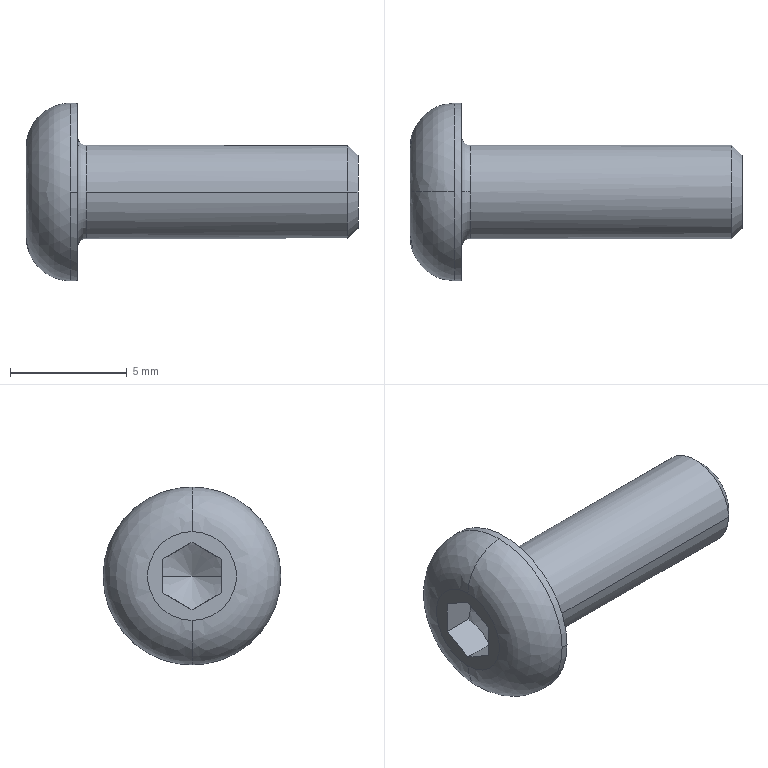Part | STEP file | ISO 7380-1 - M4 x 12 | 1 solid | 21 faces | box 14.2 x 7.6 x 7.6 mm | volume 224.738 mm3 | plane 9 | cylinder 4 | cone 4 | spline 2 | torus 2 | commonest cylinder face diameters 4 x2 7.6 x2